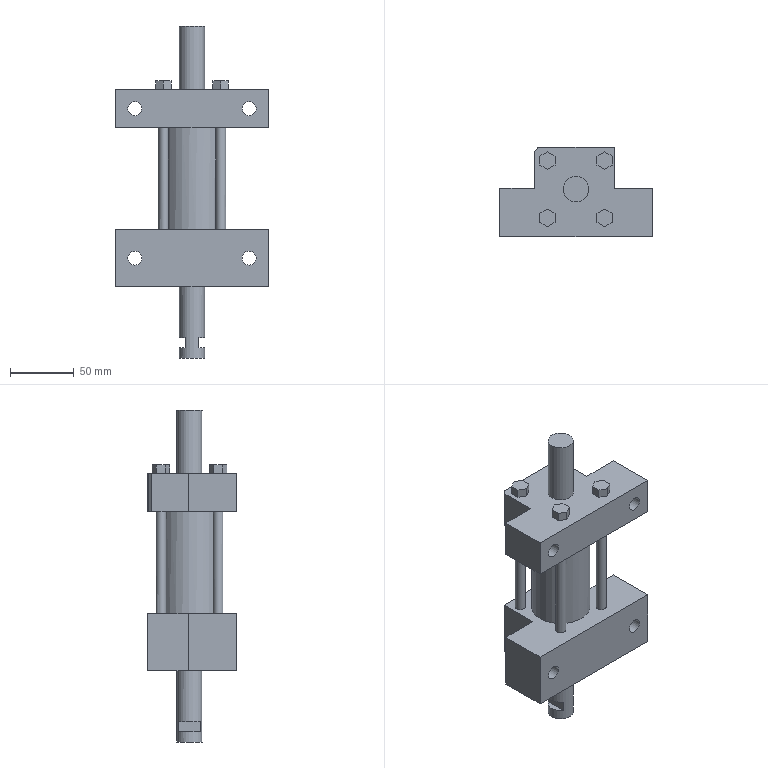Part | STEP file | solid 148 | 1 solid | 81 faces | box 120 x 70 x 261 mm | volume 645284 mm3 | plane 62 | cylinder 17 | cone 2 | commonest cylinder face diameters 8 x4 11 x4 18 x4 15 x2 20 x2 46 x1